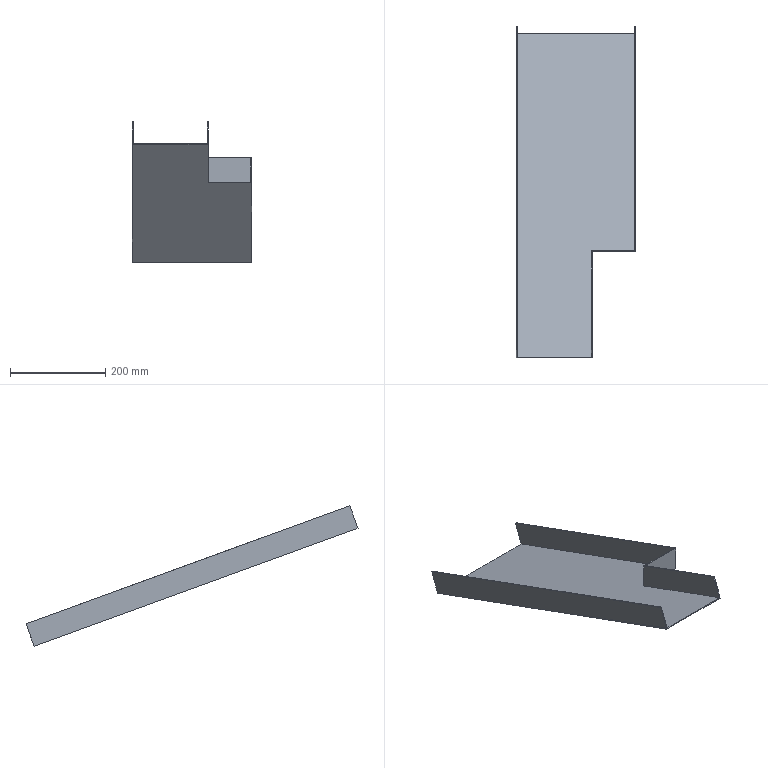Part | NX | features solid 2 | 1 solid | 14 faces | box 250 x 695.354 x 293.848 mm | volume 465781 mm3 | plane 14
STEP:
#1=CARTESIAN_POINT('',(-872.,517.,-239.51));
#2=VERTEX_POINT('',#1);
#3=CARTESIAN_POINT('',(-963.,517.,-239.51));
#4=VERTEX_POINT('',#3);
#5=CARTESIAN_POINT('',(-1225.,517.,-239.51));
#6=DIRECTION('',(1.,0.,0.));
#7=VECTOR('',#6,1000.);
#8=LINE('',#5,#7);
#9=EDGE_CURVE('',#2,#4,#8,.F.);
#10=ORIENTED_EDGE('',*,*,#9,.F.);
#11=CARTESIAN_POINT('',(-872.,971.638,-404.984));
#12=VERTEX_POINT('',#11);
#13=CARTESIAN_POINT('',(-872.,-108.795,-11.739));
#14=DIRECTION('',(0.,0.9397,-0.342));
#15=VECTOR('',#14,1000.);
#16=LINE('',#13,#15);
#17=EDGE_CURVE('',#2,#12,#16,.T.);
#18=ORIENTED_EDGE('',*,*,#17,.T.);
#19=CARTESIAN_POINT('',(-1118.,971.638,-404.984));
#20=VERTEX_POINT('',#19);
#21=CARTESIAN_POINT('',(-1100.,971.638,-404.984));
#22=DIRECTION('',(1.,0.,0.));
#23=VECTOR('',#22,1000.);
#24=LINE('',#21,#23);
#25=EDGE_CURVE('',#20,#12,#24,.T.);
#26=ORIENTED_EDGE('',*,*,#25,.F.);
#27=CARTESIAN_POINT('',(-1118.,293.385,-158.121));
#28=VERTEX_POINT('',#27);
#29=CARTESIAN_POINT('',(-1118.,-108.795,-11.739));
#30=DIRECTION('',(0.,0.9397,-0.342));
#31=VECTOR('',#30,1000.);
#32=LINE('',#29,#31);
#33=EDGE_CURVE('',#28,#20,#32,.T.);
#34=ORIENTED_EDGE('',*,*,#33,.F.);
#35=CARTESIAN_POINT('',(-963.,293.385,-158.121));
#36=VERTEX_POINT('',#35);
#37=CARTESIAN_POINT('',(-1225.,293.385,-158.121));
#38=DIRECTION('',(-1.,0.,0.));
#39=VECTOR('',#38,1000.);
#40=LINE('',#37,#39);
#41=EDGE_CURVE('',#28,#36,#40,.F.);
#42=ORIENTED_EDGE('',*,*,#41,.T.);
#43=CARTESIAN_POINT('',(-963.,-108.795,-11.739));
#44=DIRECTION('',(0.,-0.9397,0.342));
#45=VECTOR('',#44,1000.);
#46=LINE('',#43,#45);
#47=EDGE_CURVE('',#4,#36,#46,.T.);
#48=ORIENTED_EDGE('',*,*,#47,.F.);
#49=EDGE_LOOP('',(#10,#18,#26,#34,#42,#48));
#50=FACE_BOUND('',#49,.T.);
#51=CARTESIAN_POINT('',(-1225.,-108.795,-11.739));
#52=DIRECTION('',(0.,-0.342,-0.9397));
#53=DIRECTION('',(0.,0.9397,-0.342));
#54=AXIS2_PLACEMENT_3D('',#51,#52,#53);
#55=PLANE('',#54);
#56=ADVANCED_FACE('',(#50),#55,.F.);
#57=CARTESIAN_POINT('',(-961.,515.,-240.91));
#58=VERTEX_POINT('',#57);
#59=CARTESIAN_POINT('',(-961.,515.,-187.701));
#60=VERTEX_POINT('',#59);
#61=CARTESIAN_POINT('',(-961.,515.,-240.91));
#62=DIRECTION('',(0.,0.,-1.));
#63=VECTOR('',#62,1000.);
#64=LINE('',#61,#63);
#65=EDGE_CURVE('',#58,#60,#64,.F.);
#66=ORIENTED_EDGE('',*,*,#65,.T.);
#67=CARTESIAN_POINT('',(-961.,309.802,-113.015));
#68=VERTEX_POINT('',#67);
#69=CARTESIAN_POINT('',(-961.,532.101,-193.926));
#70=DIRECTION('',(0.,-0.9397,0.342));
#71=VECTOR('',#70,1000.);
#72=LINE('',#69,#71);
#73=EDGE_CURVE('',#60,#68,#72,.T.);
#74=ORIENTED_EDGE('',*,*,#73,.T.);
#75=CARTESIAN_POINT('',(-961.,292.701,-160.));
#76=VERTEX_POINT('',#75);
#77=CARTESIAN_POINT('',(-961.,292.701,-160.));
#78=DIRECTION('',(0.,0.342,0.9397));
#79=VECTOR('',#78,1000.);
#80=LINE('',#77,#79);
#81=EDGE_CURVE('',#76,#68,#80,.T.);
#82=ORIENTED_EDGE('',*,*,#81,.F.);
#83=CARTESIAN_POINT('',(-961.,-109.479,-13.618));
#84=DIRECTION('',(0.,-0.9397,0.342));
#85=VECTOR('',#84,1000.);
#86=LINE('',#83,#85);
#87=EDGE_CURVE('',#58,#76,#86,.T.);
#88=ORIENTED_EDGE('',*,*,#87,.F.);
#89=EDGE_LOOP('',(#66,#74,#82,#88));
#90=FACE_BOUND('',#89,.T.);
#91=CARTESIAN_POINT('',(-961.,-109.479,-13.618));
#92=DIRECTION('',(-1.,0.,0.));
#93=DIRECTION('',(0.,0.,1.));
#94=AXIS2_PLACEMENT_3D('',#91,#92,#93);
#95=PLANE('',#94);
#96=ADVANCED_FACE('',(#90),#95,.F.);
#97=ORIENTED_EDGE('',*,*,#17,.F.);
#98=CARTESIAN_POINT('',(-872.,517.,-188.429));
#99=VERTEX_POINT('',#98);
#100=CARTESIAN_POINT('',(-872.,517.,-193.926));
#101=DIRECTION('',(0.,0.,-1.));
#102=VECTOR('',#101,1000.);
#103=LINE('',#100,#102);
#104=EDGE_CURVE('',#2,#99,#103,.F.);
#105=ORIENTED_EDGE('',*,*,#104,.T.);
#106=CARTESIAN_POINT('',(-872.,988.055,-359.879));
#107=VERTEX_POINT('',#106);
#108=CARTESIAN_POINT('',(-872.,532.101,-193.926));
#109=DIRECTION('',(0.,0.9397,-0.342));
#110=VECTOR('',#109,1000.);
#111=LINE('',#108,#110);
#112=EDGE_CURVE('',#99,#107,#111,.T.);
#113=ORIENTED_EDGE('',*,*,#112,.T.);
#114=CARTESIAN_POINT('',(-872.,988.055,-359.879));
#115=DIRECTION('',(0.,-0.342,-0.9397));
#116=VECTOR('',#115,1000.);
#117=LINE('',#114,#116);
#118=EDGE_CURVE('',#107,#12,#117,.T.);
#119=ORIENTED_EDGE('',*,*,#118,.T.);
#120=EDGE_LOOP('',(#97,#105,#113,#119));
#121=FACE_BOUND('',#120,.T.);
#122=CARTESIAN_POINT('',(-872.,532.101,-193.926));
#123=DIRECTION('',(-1.,0.,0.));
#124=DIRECTION('',(0.,0.,1.));
#125=AXIS2_PLACEMENT_3D('',#122,#123,#124);
#126=PLANE('',#125);
#127=ADVANCED_FACE('',(#121),#126,.T.);
#128=CARTESIAN_POINT('',(-1120.,970.954,-406.864));
#129=VERTEX_POINT('',#128);
#130=CARTESIAN_POINT('',(-1120.,988.055,-359.879));
#131=VERTEX_POINT('',#130);
#132=CARTESIAN_POINT('',(-1120.,970.954,-406.864));
#133=DIRECTION('',(0.,0.342,0.9397));
#134=VECTOR('',#133,1000.);
#135=LINE('',#132,#134);
#136=EDGE_CURVE('',#129,#131,#135,.T.);
#137=ORIENTED_EDGE('',*,*,#136,.T.);
#138=CARTESIAN_POINT('',(-1118.,988.055,-359.879));
#139=VERTEX_POINT('',#138);
#140=CARTESIAN_POINT('',(-1120.,988.055,-359.879));
#141=DIRECTION('',(1.,0.,0.));
#142=VECTOR('',#141,1000.);
#143=LINE('',#140,#142);
#144=EDGE_CURVE('',#131,#139,#143,.T.);
#145=ORIENTED_EDGE('',*,*,#144,.T.);
#146=CARTESIAN_POINT('',(-1118.,988.055,-359.879));
#147=DIRECTION('',(0.,-0.342,-0.9397));
#148=VECTOR('',#147,1000.);
#149=LINE('',#146,#148);
#150=EDGE_CURVE('',#139,#20,#149,.T.);
#151=ORIENTED_EDGE('',*,*,#150,.T.);
#152=ORIENTED_EDGE('',*,*,#25,.T.);
#153=ORIENTED_EDGE('',*,*,#118,.F.);
#154=CARTESIAN_POINT('',(-870.,988.055,-359.879));
#155=VERTEX_POINT('',#154);
#156=CARTESIAN_POINT('',(-870.,988.055,-359.879));
#157=DIRECTION('',(1.,0.,0.));
#158=VECTOR('',#157,1000.);
#159=LINE('',#156,#158);
#160=EDGE_CURVE('',#155,#107,#159,.F.);
#161=ORIENTED_EDGE('',*,*,#160,.F.);
#162=CARTESIAN_POINT('',(-870.,970.954,-406.864));
#163=VERTEX_POINT('',#162);
#164=CARTESIAN_POINT('',(-870.,970.954,-406.864));
#165=DIRECTION('',(0.,0.342,0.9397));
#166=VECTOR('',#165,1000.);
#167=LINE('',#164,#166);
#168=EDGE_CURVE('',#163,#155,#167,.T.);
#169=ORIENTED_EDGE('',*,*,#168,.F.);
#170=CARTESIAN_POINT('',(-1100.,970.954,-406.864));
#171=DIRECTION('',(1.,0.,0.));
#172=VECTOR('',#171,1000.);
#173=LINE('',#170,#172);
#174=EDGE_CURVE('',#129,#163,#173,.T.);
#175=ORIENTED_EDGE('',*,*,#174,.F.);
#176=EDGE_LOOP('',(#137,#145,#151,#152,#153,#161,#169,#175));
#177=FACE_BOUND('',#176,.T.);
#178=CARTESIAN_POINT('',(-1100.,970.954,-406.864));
#179=DIRECTION('',(0.,-0.9397,0.342));
#180=DIRECTION('',(0.,-0.342,-0.9397));
#181=AXIS2_PLACEMENT_3D('',#178,#179,#180);
#182=PLANE('',#181);
#183=ADVANCED_FACE('',(#177),#182,.F.);
#184=CARTESIAN_POINT('',(-1120.,292.701,-160.));
#185=VERTEX_POINT('',#184);
#186=CARTESIAN_POINT('',(-1120.,309.802,-113.015));
#187=VERTEX_POINT('',#186);
#188=CARTESIAN_POINT('',(-1120.,292.701,-160.));
#189=DIRECTION('',(0.,0.342,0.9397));
#190=VECTOR('',#189,1000.);
#191=LINE('',#188,#190);
#192=EDGE_CURVE('',#185,#187,#191,.T.);
#193=ORIENTED_EDGE('',*,*,#192,.T.);
#194=CARTESIAN_POINT('',(-1120.,309.802,-113.015));
#195=DIRECTION('',(0.,0.9397,-0.342));
#196=VECTOR('',#195,1000.);
#197=LINE('',#194,#196);
#198=EDGE_CURVE('',#187,#131,#197,.T.);
#199=ORIENTED_EDGE('',*,*,#198,.T.);
#200=ORIENTED_EDGE('',*,*,#136,.F.);
#201=CARTESIAN_POINT('',(-1120.,-109.479,-13.618));
#202=DIRECTION('',(0.,-0.9397,0.342));
#203=VECTOR('',#202,1000.);
#204=LINE('',#201,#203);
#205=EDGE_CURVE('',#185,#129,#204,.F.);
#206=ORIENTED_EDGE('',*,*,#205,.F.);
#207=EDGE_LOOP('',(#193,#199,#200,#206));
#208=FACE_BOUND('',#207,.T.);
#209=CARTESIAN_POINT('',(-1120.,-109.479,-13.618));
#210=DIRECTION('',(1.,0.,0.));
#211=DIRECTION('',(0.,0.,-1.));
#212=AXIS2_PLACEMENT_3D('',#209,#210,#211);
#213=PLANE('',#212);
#214=ADVANCED_FACE('',(#208),#213,.F.);
#215=CARTESIAN_POINT('',(-1225.,292.701,-160.));
#216=DIRECTION('',(-1.,0.,0.));
#217=VECTOR('',#216,1000.);
#218=LINE('',#215,#217);
#219=EDGE_CURVE('',#185,#76,#218,.F.);
#220=ORIENTED_EDGE('',*,*,#219,.T.);
#221=ORIENTED_EDGE('',*,*,#81,.T.);
#222=CARTESIAN_POINT('',(-963.,309.802,-113.015));
#223=VERTEX_POINT('',#222);
#224=CARTESIAN_POINT('',(-961.,309.802,-113.015));
#225=DIRECTION('',(1.,0.,0.));
#226=VECTOR('',#225,1000.);
#227=LINE('',#224,#226);
#228=EDGE_CURVE('',#68,#223,#227,.F.);
#229=ORIENTED_EDGE('',*,*,#228,.T.);
#230=CARTESIAN_POINT('',(-963.,309.802,-113.015));
#231=DIRECTION('',(0.,-0.342,-0.9397));
#232=VECTOR('',#231,1000.);
#233=LINE('',#230,#232);
#234=EDGE_CURVE('',#223,#36,#233,.T.);
#235=ORIENTED_EDGE('',*,*,#234,.T.);
#236=ORIENTED_EDGE('',*,*,#41,.F.);
#237=CARTESIAN_POINT('',(-1118.,309.802,-113.015));
#238=VERTEX_POINT('',#237);
#239=CARTESIAN_POINT('',(-1118.,309.802,-113.015));
#240=DIRECTION('',(0.,-0.342,-0.9397));
#241=VECTOR('',#240,1000.);
#242=LINE('',#239,#241);
#243=EDGE_CURVE('',#238,#28,#242,.T.);
#244=ORIENTED_EDGE('',*,*,#243,.F.);
#245=CARTESIAN_POINT('',(-1120.,309.802,-113.015));
#246=DIRECTION('',(1.,0.,0.));
#247=VECTOR('',#246,1000.);
#248=LINE('',#245,#247);
#249=EDGE_CURVE('',#187,#238,#248,.T.);
#250=ORIENTED_EDGE('',*,*,#249,.F.);
#251=ORIENTED_EDGE('',*,*,#192,.F.);
#252=EDGE_LOOP('',(#220,#221,#229,#235,#236,#244,#250,#251));
#253=FACE_BOUND('',#252,.T.);
#254=CARTESIAN_POINT('',(-1225.,292.701,-160.));
#255=DIRECTION('',(0.,-0.9397,0.342));
#256=DIRECTION('',(0.,-0.342,-0.9397));
#257=AXIS2_PLACEMENT_3D('',#254,#255,#256);
#258=PLANE('',#257);
#259=ADVANCED_FACE('',(#253),#258,.T.);
#260=CARTESIAN_POINT('',(-870.,515.,-187.701));
#261=VERTEX_POINT('',#260);
#262=CARTESIAN_POINT('',(-870.,532.101,-193.926));
#263=DIRECTION('',(0.,0.9397,-0.342));
#264=VECTOR('',#263,1000.);
#265=LINE('',#262,#264);
#266=EDGE_CURVE('',#261,#155,#265,.T.);
#267=ORIENTED_EDGE('',*,*,#266,.F.);
#268=CARTESIAN_POINT('',(-870.,515.,-240.91));
#269=VERTEX_POINT('',#268);
#270=CARTESIAN_POINT('',(-870.,515.,-240.91));
#271=DIRECTION('',(0.,0.,-1.));
#272=VECTOR('',#271,1000.);
#273=LINE('',#270,#272);
#274=EDGE_CURVE('',#269,#261,#273,.F.);
#275=ORIENTED_EDGE('',*,*,#274,.F.);
#276=CARTESIAN_POINT('',(-870.,-109.479,-13.618));
#277=DIRECTION('',(0.,0.9397,-0.342));
#278=VECTOR('',#277,1000.);
#279=LINE('',#276,#278);
#280=EDGE_CURVE('',#269,#163,#279,.T.);
#281=ORIENTED_EDGE('',*,*,#280,.T.);
#282=ORIENTED_EDGE('',*,*,#168,.T.);
#283=EDGE_LOOP('',(#267,#275,#281,#282));
#284=FACE_BOUND('',#283,.T.);
#285=CARTESIAN_POINT('',(-870.,-109.479,-13.618));
#286=DIRECTION('',(1.,0.,0.));
#287=DIRECTION('',(0.,0.,-1.));
#288=AXIS2_PLACEMENT_3D('',#285,#286,#287);
#289=PLANE('',#288);
#290=ADVANCED_FACE('',(#284),#289,.T.);
#291=ORIENTED_EDGE('',*,*,#174,.T.);
#292=ORIENTED_EDGE('',*,*,#280,.F.);
#293=CARTESIAN_POINT('',(-1225.,515.,-240.91));
#294=DIRECTION('',(-1.,0.,0.));
#295=VECTOR('',#294,1000.);
#296=LINE('',#293,#295);
#297=EDGE_CURVE('',#269,#58,#296,.T.);
#298=ORIENTED_EDGE('',*,*,#297,.T.);
#299=ORIENTED_EDGE('',*,*,#87,.T.);
#300=ORIENTED_EDGE('',*,*,#219,.F.);
#301=ORIENTED_EDGE('',*,*,#205,.T.);
#302=EDGE_LOOP('',(#291,#292,#298,#299,#300,#301));
#303=FACE_BOUND('',#302,.T.);
#304=CARTESIAN_POINT('',(-1225.,-109.479,-13.618));
#305=DIRECTION('',(0.,-0.342,-0.9397));
#306=DIRECTION('',(0.,0.9397,-0.342));
#307=AXIS2_PLACEMENT_3D('',#304,#305,#306);
#308=PLANE('',#307);
#309=ADVANCED_FACE('',(#303),#308,.T.);
#310=CARTESIAN_POINT('',(-963.,517.,-188.429));
#311=VERTEX_POINT('',#310);
#312=CARTESIAN_POINT('',(-961.,517.,-188.429));
#313=DIRECTION('',(-1.,0.,0.));
#314=VECTOR('',#313,1000.);
#315=LINE('',#312,#314);
#316=EDGE_CURVE('',#99,#311,#315,.T.);
#317=ORIENTED_EDGE('',*,*,#316,.F.);
#318=ORIENTED_EDGE('',*,*,#104,.F.);
#319=ORIENTED_EDGE('',*,*,#9,.T.);
#320=CARTESIAN_POINT('',(-963.,517.,-193.926));
#321=DIRECTION('',(0.,0.,1.));
#322=VECTOR('',#321,1000.);
#323=LINE('',#320,#322);
#324=EDGE_CURVE('',#311,#4,#323,.F.);
#325=ORIENTED_EDGE('',*,*,#324,.F.);
#326=EDGE_LOOP('',(#317,#318,#319,#325));
#327=FACE_BOUND('',#326,.T.);
#328=CARTESIAN_POINT('',(-870.,517.,-240.91));
#329=DIRECTION('',(0.,1.,0.));
#330=DIRECTION('',(-1.,0.,0.));
#331=AXIS2_PLACEMENT_3D('',#328,#329,#330);
#332=PLANE('',#331);
#333=ADVANCED_FACE('',(#327),#332,.T.);
#334=ORIENTED_EDGE('',*,*,#324,.T.);
#335=ORIENTED_EDGE('',*,*,#47,.T.);
#336=ORIENTED_EDGE('',*,*,#234,.F.);
#337=CARTESIAN_POINT('',(-963.,532.101,-193.926));
#338=DIRECTION('',(0.,-0.9397,0.342));
#339=VECTOR('',#338,1000.);
#340=LINE('',#337,#339);
#341=EDGE_CURVE('',#311,#223,#340,.T.);
#342=ORIENTED_EDGE('',*,*,#341,.F.);
#343=EDGE_LOOP('',(#334,#335,#336,#342));
#344=FACE_BOUND('',#343,.T.);
#345=CARTESIAN_POINT('',(-963.,532.101,-193.926));
#346=DIRECTION('',(1.,0.,0.));
#347=DIRECTION('',(0.,0.,-1.));
#348=AXIS2_PLACEMENT_3D('',#345,#346,#347);
#349=PLANE('',#348);
#350=ADVANCED_FACE('',(#344),#349,.F.);
#351=ORIENTED_EDGE('',*,*,#316,.T.);
#352=ORIENTED_EDGE('',*,*,#341,.T.);
#353=ORIENTED_EDGE('',*,*,#228,.F.);
#354=ORIENTED_EDGE('',*,*,#73,.F.);
#355=CARTESIAN_POINT('',(-870.,515.,-187.701));
#356=DIRECTION('',(-1.,0.,0.));
#357=VECTOR('',#356,1000.);
#358=LINE('',#355,#357);
#359=EDGE_CURVE('',#261,#60,#358,.T.);
#360=ORIENTED_EDGE('',*,*,#359,.F.);
#361=ORIENTED_EDGE('',*,*,#266,.T.);
#362=ORIENTED_EDGE('',*,*,#160,.T.);
#363=ORIENTED_EDGE('',*,*,#112,.F.);
#364=EDGE_LOOP('',(#351,#352,#353,#354,#360,#361,#362,#363));
#365=FACE_BOUND('',#364,.T.);
#366=CARTESIAN_POINT('',(-961.,532.101,-193.926));
#367=DIRECTION('',(0.,0.342,0.9397));
#368=DIRECTION('',(0.,-0.9397,0.342));
#369=AXIS2_PLACEMENT_3D('',#366,#367,#368);
#370=PLANE('',#369);
#371=ADVANCED_FACE('',(#365),#370,.T.);
#372=ORIENTED_EDGE('',*,*,#243,.T.);
#373=ORIENTED_EDGE('',*,*,#33,.T.);
#374=ORIENTED_EDGE('',*,*,#150,.F.);
#375=CARTESIAN_POINT('',(-1118.,309.802,-113.015));
#376=DIRECTION('',(0.,0.9397,-0.342));
#377=VECTOR('',#376,1000.);
#378=LINE('',#375,#377);
#379=EDGE_CURVE('',#238,#139,#378,.T.);
#380=ORIENTED_EDGE('',*,*,#379,.F.);
#381=EDGE_LOOP('',(#372,#373,#374,#380));
#382=FACE_BOUND('',#381,.T.);
#383=CARTESIAN_POINT('',(-1118.,309.802,-113.015));
#384=DIRECTION('',(-1.,0.,0.));
#385=DIRECTION('',(0.,0.,1.));
#386=AXIS2_PLACEMENT_3D('',#383,#384,#385);
#387=PLANE('',#386);
#388=ADVANCED_FACE('',(#382),#387,.F.);
#389=ORIENTED_EDGE('',*,*,#144,.F.);
#390=ORIENTED_EDGE('',*,*,#198,.F.);
#391=ORIENTED_EDGE('',*,*,#249,.T.);
#392=ORIENTED_EDGE('',*,*,#379,.T.);
#393=EDGE_LOOP('',(#389,#390,#391,#392));
#394=FACE_BOUND('',#393,.T.);
#395=CARTESIAN_POINT('',(-1120.,309.802,-113.015));
#396=DIRECTION('',(0.,0.342,0.9397));
#397=DIRECTION('',(0.,0.9397,-0.342));
#398=AXIS2_PLACEMENT_3D('',#395,#396,#397);
#399=PLANE('',#398);
#400=ADVANCED_FACE('',(#394),#399,.T.);
#401=ORIENTED_EDGE('',*,*,#274,.T.);
#402=ORIENTED_EDGE('',*,*,#359,.T.);
#403=ORIENTED_EDGE('',*,*,#65,.F.);
#404=ORIENTED_EDGE('',*,*,#297,.F.);
#405=EDGE_LOOP('',(#401,#402,#403,#404));
#406=FACE_BOUND('',#405,.T.);
#407=CARTESIAN_POINT('',(-870.,515.,-240.91));
#408=DIRECTION('',(0.,1.,0.));
#409=DIRECTION('',(-1.,0.,0.));
#410=AXIS2_PLACEMENT_3D('',#407,#408,#409);
#411=PLANE('',#410);
#412=ADVANCED_FACE('',(#406),#411,.F.);
#413=CLOSED_SHELL('',(#56,#96,#127,#183,#214,#259,#290,#309,#333,#350,#371,#388,#400,#412));
#414=MANIFOLD_SOLID_BREP('',#413);
#415=(LENGTH_UNIT()NAMED_UNIT(*)SI_UNIT(.MILLI.,.METRE.));
#416=UNCERTAINTY_MEASURE_WITH_UNIT(LENGTH_MEASURE(0.00001),#415,'','');
#417=(NAMED_UNIT(*)PLANE_ANGLE_UNIT()SI_UNIT($,.RADIAN.));
#418=(NAMED_UNIT(*)SI_UNIT($,.STERADIAN.)SOLID_ANGLE_UNIT());
#419=(GEOMETRIC_REPRESENTATION_CONTEXT(3)GLOBAL_UNCERTAINTY_ASSIGNED_CONTEXT((#416))GLOBAL_UNIT_ASSIGNED_CONTEXT((#415,#417,#418))REPRESENTATION_CONTEXT('',''));
#420=ADVANCED_BREP_SHAPE_REPRESENTATION('',(#414),#419);